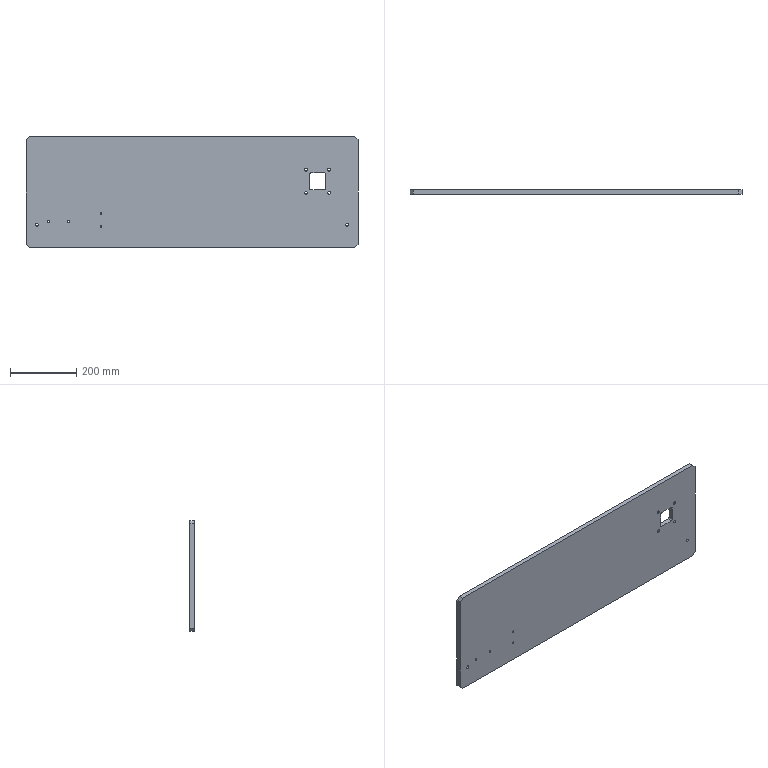Part | SolidWorks | features BaseBody 1 | 1 solid | 38 faces | box 1005 x 14 x 335 mm | volume 4668914 mm3 | cylinder 24 | plane 14 | commonest cylinder face diameters 8.5 x12 5 x4 6.8 x4 10 x4
STEP:
#1=CARTESIAN_POINT('',(470.,0.,-103.382));
#2=VERTEX_POINT('',#1);
#3=CARTESIAN_POINT('',(470.,0.,-94.882));
#4=VERTEX_POINT('',#3);
#5=CARTESIAN_POINT('',(470.,0.,-99.132));
#6=DIRECTION('',(0.,1.,0.));
#7=DIRECTION('',(0.,0.,1.));
#8=AXIS2_PLACEMENT_3D('',#5,#6,#7);
#9=CIRCLE('',#8,4.25);
#10=EDGE_CURVE('',#2,#4,#9,.T.);
#11=ORIENTED_EDGE('',*,*,#10,.F.);
#12=CARTESIAN_POINT('',(470.,14.,-103.382));
#13=VERTEX_POINT('',#12);
#14=CARTESIAN_POINT('',(470.,14.,-103.382));
#15=DIRECTION('',(0.,1.,0.));
#16=VECTOR('',#15,1000.);
#17=LINE('',#14,#16);
#18=EDGE_CURVE('',#2,#13,#17,.T.);
#19=ORIENTED_EDGE('',*,*,#18,.T.);
#20=CARTESIAN_POINT('',(470.,14.,-94.882));
#21=VERTEX_POINT('',#20);
#22=CARTESIAN_POINT('',(470.,14.,-99.132));
#23=DIRECTION('',(0.,1.,0.));
#24=DIRECTION('',(0.,0.,1.));
#25=AXIS2_PLACEMENT_3D('',#22,#23,#24);
#26=CIRCLE('',#25,4.25);
#27=EDGE_CURVE('',#13,#21,#26,.T.);
#28=ORIENTED_EDGE('',*,*,#27,.T.);
#29=CARTESIAN_POINT('',(470.,14.,-94.882));
#30=DIRECTION('',(0.,1.,0.));
#31=VECTOR('',#30,1000.);
#32=LINE('',#29,#31);
#33=EDGE_CURVE('',#4,#21,#32,.T.);
#34=ORIENTED_EDGE('',*,*,#33,.F.);
#35=EDGE_LOOP('',(#11,#19,#28,#34));
#36=FACE_OUTER_BOUND('',#35,.T.);
#37=CARTESIAN_POINT('',(470.,14.,-99.132));
#38=DIRECTION('',(0.,1.,0.));
#39=DIRECTION('',(0.,0.,1.));
#40=AXIS2_PLACEMENT_3D('',#37,#38,#39);
#41=CYLINDRICAL_SURFACE('',#40,4.25);
#42=ADVANCED_FACE('',(#36),#41,.F.);
#43=CARTESIAN_POINT('',(345.,0.,63.25));
#44=VERTEX_POINT('',#43);
#45=CARTESIAN_POINT('',(345.,0.,71.75));
#46=VERTEX_POINT('',#45);
#47=CARTESIAN_POINT('',(345.,0.,67.5));
#48=DIRECTION('',(0.,1.,0.));
#49=DIRECTION('',(0.,0.,1.));
#50=AXIS2_PLACEMENT_3D('',#47,#48,#49);
#51=CIRCLE('',#50,4.25);
#52=EDGE_CURVE('',#44,#46,#51,.T.);
#53=ORIENTED_EDGE('',*,*,#52,.F.);
#54=CARTESIAN_POINT('',(345.,14.,63.25));
#55=VERTEX_POINT('',#54);
#56=CARTESIAN_POINT('',(345.,14.,63.25));
#57=DIRECTION('',(0.,1.,0.));
#58=VECTOR('',#57,1000.);
#59=LINE('',#56,#58);
#60=EDGE_CURVE('',#44,#55,#59,.T.);
#61=ORIENTED_EDGE('',*,*,#60,.T.);
#62=CARTESIAN_POINT('',(345.,14.,71.75));
#63=VERTEX_POINT('',#62);
#64=CARTESIAN_POINT('',(345.,14.,67.5));
#65=DIRECTION('',(0.,1.,0.));
#66=DIRECTION('',(0.,0.,1.));
#67=AXIS2_PLACEMENT_3D('',#64,#65,#66);
#68=CIRCLE('',#67,4.25);
#69=EDGE_CURVE('',#55,#63,#68,.T.);
#70=ORIENTED_EDGE('',*,*,#69,.T.);
#71=CARTESIAN_POINT('',(345.,14.,71.75));
#72=DIRECTION('',(0.,1.,0.));
#73=VECTOR('',#72,1000.);
#74=LINE('',#71,#73);
#75=EDGE_CURVE('',#46,#63,#74,.T.);
#76=ORIENTED_EDGE('',*,*,#75,.F.);
#77=EDGE_LOOP('',(#53,#61,#70,#76));
#78=FACE_OUTER_BOUND('',#77,.T.);
#79=CARTESIAN_POINT('',(345.,14.,67.5));
#80=DIRECTION('',(0.,1.,0.));
#81=DIRECTION('',(0.,0.,1.));
#82=AXIS2_PLACEMENT_3D('',#79,#80,#81);
#83=CYLINDRICAL_SURFACE('',#82,4.25);
#84=ADVANCED_FACE('',(#78),#83,.F.);
#85=CARTESIAN_POINT('',(415.,0.,63.25));
#86=VERTEX_POINT('',#85);
#87=CARTESIAN_POINT('',(415.,0.,71.75));
#88=VERTEX_POINT('',#87);
#89=CARTESIAN_POINT('',(415.,0.,67.5));
#90=DIRECTION('',(0.,1.,0.));
#91=DIRECTION('',(0.,0.,1.));
#92=AXIS2_PLACEMENT_3D('',#89,#90,#91);
#93=CIRCLE('',#92,4.25);
#94=EDGE_CURVE('',#86,#88,#93,.T.);
#95=ORIENTED_EDGE('',*,*,#94,.F.);
#96=CARTESIAN_POINT('',(415.,14.,63.25));
#97=VERTEX_POINT('',#96);
#98=CARTESIAN_POINT('',(415.,14.,63.25));
#99=DIRECTION('',(0.,1.,0.));
#100=VECTOR('',#99,1000.);
#101=LINE('',#98,#100);
#102=EDGE_CURVE('',#86,#97,#101,.T.);
#103=ORIENTED_EDGE('',*,*,#102,.T.);
#104=CARTESIAN_POINT('',(415.,14.,71.75));
#105=VERTEX_POINT('',#104);
#106=CARTESIAN_POINT('',(415.,14.,67.5));
#107=DIRECTION('',(0.,1.,0.));
#108=DIRECTION('',(0.,0.,1.));
#109=AXIS2_PLACEMENT_3D('',#106,#107,#108);
#110=CIRCLE('',#109,4.25);
#111=EDGE_CURVE('',#97,#105,#110,.T.);
#112=ORIENTED_EDGE('',*,*,#111,.T.);
#113=CARTESIAN_POINT('',(415.,14.,71.75));
#114=DIRECTION('',(0.,1.,0.));
#115=VECTOR('',#114,1000.);
#116=LINE('',#113,#115);
#117=EDGE_CURVE('',#88,#105,#116,.T.);
#118=ORIENTED_EDGE('',*,*,#117,.F.);
#119=EDGE_LOOP('',(#95,#103,#112,#118));
#120=FACE_OUTER_BOUND('',#119,.T.);
#121=CARTESIAN_POINT('',(415.,14.,67.5));
#122=DIRECTION('',(0.,1.,0.));
#123=DIRECTION('',(0.,0.,1.));
#124=AXIS2_PLACEMENT_3D('',#121,#122,#123);
#125=CYLINDRICAL_SURFACE('',#124,4.25);
#126=ADVANCED_FACE('',(#120),#125,.F.);
#127=CARTESIAN_POINT('',(415.,0.,-6.75));
#128=VERTEX_POINT('',#127);
#129=CARTESIAN_POINT('',(415.,0.,1.75));
#130=VERTEX_POINT('',#129);
#131=CARTESIAN_POINT('',(415.,0.,-2.5));
#132=DIRECTION('',(0.,1.,0.));
#133=DIRECTION('',(0.,0.,1.));
#134=AXIS2_PLACEMENT_3D('',#131,#132,#133);
#135=CIRCLE('',#134,4.25);
#136=EDGE_CURVE('',#128,#130,#135,.T.);
#137=ORIENTED_EDGE('',*,*,#136,.F.);
#138=CARTESIAN_POINT('',(415.,14.,-6.75));
#139=VERTEX_POINT('',#138);
#140=CARTESIAN_POINT('',(415.,14.,-6.75));
#141=DIRECTION('',(0.,1.,0.));
#142=VECTOR('',#141,1000.);
#143=LINE('',#140,#142);
#144=EDGE_CURVE('',#128,#139,#143,.T.);
#145=ORIENTED_EDGE('',*,*,#144,.T.);
#146=CARTESIAN_POINT('',(415.,14.,1.75));
#147=VERTEX_POINT('',#146);
#148=CARTESIAN_POINT('',(415.,14.,-2.5));
#149=DIRECTION('',(0.,1.,0.));
#150=DIRECTION('',(0.,0.,1.));
#151=AXIS2_PLACEMENT_3D('',#148,#149,#150);
#152=CIRCLE('',#151,4.25);
#153=EDGE_CURVE('',#139,#147,#152,.T.);
#154=ORIENTED_EDGE('',*,*,#153,.T.);
#155=CARTESIAN_POINT('',(415.,14.,1.75));
#156=DIRECTION('',(0.,1.,0.));
#157=VECTOR('',#156,1000.);
#158=LINE('',#155,#157);
#159=EDGE_CURVE('',#130,#147,#158,.T.);
#160=ORIENTED_EDGE('',*,*,#159,.F.);
#161=EDGE_LOOP('',(#137,#145,#154,#160));
#162=FACE_OUTER_BOUND('',#161,.T.);
#163=CARTESIAN_POINT('',(415.,14.,-2.5));
#164=DIRECTION('',(0.,1.,0.));
#165=DIRECTION('',(0.,0.,1.));
#166=AXIS2_PLACEMENT_3D('',#163,#164,#165);
#167=CYLINDRICAL_SURFACE('',#166,4.25);
#168=ADVANCED_FACE('',(#162),#167,.F.);
#169=CARTESIAN_POINT('',(345.,0.,-6.75));
#170=VERTEX_POINT('',#169);
#171=CARTESIAN_POINT('',(345.,0.,1.75));
#172=VERTEX_POINT('',#171);
#173=CARTESIAN_POINT('',(345.,0.,-2.5));
#174=DIRECTION('',(0.,1.,0.));
#175=DIRECTION('',(0.,0.,1.));
#176=AXIS2_PLACEMENT_3D('',#173,#174,#175);
#177=CIRCLE('',#176,4.25);
#178=EDGE_CURVE('',#170,#172,#177,.T.);
#179=ORIENTED_EDGE('',*,*,#178,.F.);
#180=CARTESIAN_POINT('',(345.,14.,-6.75));
#181=VERTEX_POINT('',#180);
#182=CARTESIAN_POINT('',(345.,14.,-6.75));
#183=DIRECTION('',(0.,1.,0.));
#184=VECTOR('',#183,1000.);
#185=LINE('',#182,#184);
#186=EDGE_CURVE('',#170,#181,#185,.T.);
#187=ORIENTED_EDGE('',*,*,#186,.T.);
#188=CARTESIAN_POINT('',(345.,14.,1.75));
#189=VERTEX_POINT('',#188);
#190=CARTESIAN_POINT('',(345.,14.,-2.5));
#191=DIRECTION('',(0.,1.,0.));
#192=DIRECTION('',(0.,0.,1.));
#193=AXIS2_PLACEMENT_3D('',#190,#191,#192);
#194=CIRCLE('',#193,4.25);
#195=EDGE_CURVE('',#181,#189,#194,.T.);
#196=ORIENTED_EDGE('',*,*,#195,.T.);
#197=CARTESIAN_POINT('',(345.,14.,1.75));
#198=DIRECTION('',(0.,1.,0.));
#199=VECTOR('',#198,1000.);
#200=LINE('',#197,#199);
#201=EDGE_CURVE('',#172,#189,#200,.T.);
#202=ORIENTED_EDGE('',*,*,#201,.F.);
#203=EDGE_LOOP('',(#179,#187,#196,#202));
#204=FACE_OUTER_BOUND('',#203,.T.);
#205=CARTESIAN_POINT('',(345.,14.,-2.5));
#206=DIRECTION('',(0.,1.,0.));
#207=DIRECTION('',(0.,0.,1.));
#208=AXIS2_PLACEMENT_3D('',#205,#206,#207);
#209=CYLINDRICAL_SURFACE('',#208,4.25);
#210=ADVANCED_FACE('',(#204),#209,.F.);
#211=CARTESIAN_POINT('',(-470.,0.,-103.382));
#212=VERTEX_POINT('',#211);
#213=CARTESIAN_POINT('',(-470.,0.,-94.882));
#214=VERTEX_POINT('',#213);
#215=CARTESIAN_POINT('',(-470.,0.,-99.132));
#216=DIRECTION('',(0.,1.,0.));
#217=DIRECTION('',(0.,0.,1.));
#218=AXIS2_PLACEMENT_3D('',#215,#216,#217);
#219=CIRCLE('',#218,4.25);
#220=EDGE_CURVE('',#212,#214,#219,.T.);
#221=ORIENTED_EDGE('',*,*,#220,.F.);
#222=CARTESIAN_POINT('',(-470.,14.,-103.382));
#223=VERTEX_POINT('',#222);
#224=CARTESIAN_POINT('',(-470.,14.,-103.382));
#225=DIRECTION('',(0.,1.,0.));
#226=VECTOR('',#225,1000.);
#227=LINE('',#224,#226);
#228=EDGE_CURVE('',#212,#223,#227,.T.);
#229=ORIENTED_EDGE('',*,*,#228,.T.);
#230=CARTESIAN_POINT('',(-470.,14.,-94.882));
#231=VERTEX_POINT('',#230);
#232=CARTESIAN_POINT('',(-470.,14.,-99.132));
#233=DIRECTION('',(0.,1.,0.));
#234=DIRECTION('',(0.,0.,1.));
#235=AXIS2_PLACEMENT_3D('',#232,#233,#234);
#236=CIRCLE('',#235,4.25);
#237=EDGE_CURVE('',#223,#231,#236,.T.);
#238=ORIENTED_EDGE('',*,*,#237,.T.);
#239=CARTESIAN_POINT('',(-470.,14.,-94.882));
#240=DIRECTION('',(0.,1.,0.));
#241=VECTOR('',#240,1000.);
#242=LINE('',#239,#241);
#243=EDGE_CURVE('',#214,#231,#242,.T.);
#244=ORIENTED_EDGE('',*,*,#243,.F.);
#245=EDGE_LOOP('',(#221,#229,#238,#244));
#246=FACE_OUTER_BOUND('',#245,.T.);
#247=CARTESIAN_POINT('',(-470.,14.,-99.132));
#248=DIRECTION('',(0.,1.,0.));
#249=DIRECTION('',(0.,0.,1.));
#250=AXIS2_PLACEMENT_3D('',#247,#248,#249);
#251=CYLINDRICAL_SURFACE('',#250,4.25);
#252=ADVANCED_FACE('',(#246),#251,.F.);
#253=CARTESIAN_POINT('',(-375.,0.,-92.4));
#254=VERTEX_POINT('',#253);
#255=CARTESIAN_POINT('',(-375.,0.,-85.6));
#256=VERTEX_POINT('',#255);
#257=CARTESIAN_POINT('',(-375.,0.,-89.));
#258=DIRECTION('',(0.,1.,0.));
#259=DIRECTION('',(0.,0.,1.));
#260=AXIS2_PLACEMENT_3D('',#257,#258,#259);
#261=CIRCLE('',#260,3.4);
#262=EDGE_CURVE('',#254,#256,#261,.T.);
#263=ORIENTED_EDGE('',*,*,#262,.F.);
#264=CARTESIAN_POINT('',(-375.,14.,-92.4));
#265=VERTEX_POINT('',#264);
#266=CARTESIAN_POINT('',(-375.,14.,-92.4));
#267=DIRECTION('',(0.,1.,0.));
#268=VECTOR('',#267,1000.);
#269=LINE('',#266,#268);
#270=EDGE_CURVE('',#254,#265,#269,.T.);
#271=ORIENTED_EDGE('',*,*,#270,.T.);
#272=CARTESIAN_POINT('',(-375.,14.,-85.6));
#273=VERTEX_POINT('',#272);
#274=CARTESIAN_POINT('',(-375.,14.,-89.));
#275=DIRECTION('',(0.,1.,0.));
#276=DIRECTION('',(0.,0.,1.));
#277=AXIS2_PLACEMENT_3D('',#274,#275,#276);
#278=CIRCLE('',#277,3.4);
#279=EDGE_CURVE('',#265,#273,#278,.T.);
#280=ORIENTED_EDGE('',*,*,#279,.T.);
#281=CARTESIAN_POINT('',(-375.,14.,-85.6));
#282=DIRECTION('',(0.,1.,0.));
#283=VECTOR('',#282,1000.);
#284=LINE('',#281,#283);
#285=EDGE_CURVE('',#256,#273,#284,.T.);
#286=ORIENTED_EDGE('',*,*,#285,.F.);
#287=EDGE_LOOP('',(#263,#271,#280,#286));
#288=FACE_OUTER_BOUND('',#287,.T.);
#289=CARTESIAN_POINT('',(-375.,14.,-89.));
#290=DIRECTION('',(0.,1.,0.));
#291=DIRECTION('',(0.,0.,1.));
#292=AXIS2_PLACEMENT_3D('',#289,#290,#291);
#293=CYLINDRICAL_SURFACE('',#292,3.4);
#294=ADVANCED_FACE('',(#288),#293,.F.);
#295=CARTESIAN_POINT('',(-435.,0.,-92.4));
#296=VERTEX_POINT('',#295);
#297=CARTESIAN_POINT('',(-435.,0.,-85.6));
#298=VERTEX_POINT('',#297);
#299=CARTESIAN_POINT('',(-435.,0.,-89.));
#300=DIRECTION('',(0.,1.,0.));
#301=DIRECTION('',(0.,0.,1.));
#302=AXIS2_PLACEMENT_3D('',#299,#300,#301);
#303=CIRCLE('',#302,3.4);
#304=EDGE_CURVE('',#296,#298,#303,.T.);
#305=ORIENTED_EDGE('',*,*,#304,.F.);
#306=CARTESIAN_POINT('',(-435.,14.,-92.4));
#307=VERTEX_POINT('',#306);
#308=CARTESIAN_POINT('',(-435.,14.,-92.4));
#309=DIRECTION('',(0.,1.,0.));
#310=VECTOR('',#309,1000.);
#311=LINE('',#308,#310);
#312=EDGE_CURVE('',#296,#307,#311,.T.);
#313=ORIENTED_EDGE('',*,*,#312,.T.);
#314=CARTESIAN_POINT('',(-435.,14.,-85.6));
#315=VERTEX_POINT('',#314);
#316=CARTESIAN_POINT('',(-435.,14.,-89.));
#317=DIRECTION('',(0.,1.,0.));
#318=DIRECTION('',(0.,0.,1.));
#319=AXIS2_PLACEMENT_3D('',#316,#317,#318);
#320=CIRCLE('',#319,3.4);
#321=EDGE_CURVE('',#307,#315,#320,.T.);
#322=ORIENTED_EDGE('',*,*,#321,.T.);
#323=CARTESIAN_POINT('',(-435.,14.,-85.6));
#324=DIRECTION('',(0.,1.,0.));
#325=VECTOR('',#324,1000.);
#326=LINE('',#323,#325);
#327=EDGE_CURVE('',#298,#315,#326,.T.);
#328=ORIENTED_EDGE('',*,*,#327,.F.);
#329=EDGE_LOOP('',(#305,#313,#322,#328));
#330=FACE_OUTER_BOUND('',#329,.T.);
#331=CARTESIAN_POINT('',(-435.,14.,-89.));
#332=DIRECTION('',(0.,1.,0.));
#333=DIRECTION('',(0.,0.,1.));
#334=AXIS2_PLACEMENT_3D('',#331,#332,#333);
#335=CYLINDRICAL_SURFACE('',#334,3.4);
#336=ADVANCED_FACE('',(#330),#335,.F.);
#337=CARTESIAN_POINT('',(-275.5,0.,-67.));
#338=VERTEX_POINT('',#337);
#339=CARTESIAN_POINT('',(-275.5,0.,-62.));
#340=VERTEX_POINT('',#339);
#341=CARTESIAN_POINT('',(-275.5,0.,-64.5));
#342=DIRECTION('',(0.,1.,0.));
#343=DIRECTION('',(0.,0.,1.));
#344=AXIS2_PLACEMENT_3D('',#341,#342,#343);
#345=CIRCLE('',#344,2.5);
#346=EDGE_CURVE('',#338,#340,#345,.T.);
#347=ORIENTED_EDGE('',*,*,#346,.F.);
#348=CARTESIAN_POINT('',(-275.5,14.,-67.));
#349=VERTEX_POINT('',#348);
#350=CARTESIAN_POINT('',(-275.5,14.,-67.));
#351=DIRECTION('',(0.,1.,0.));
#352=VECTOR('',#351,1000.);
#353=LINE('',#350,#352);
#354=EDGE_CURVE('',#338,#349,#353,.T.);
#355=ORIENTED_EDGE('',*,*,#354,.T.);
#356=CARTESIAN_POINT('',(-275.5,14.,-62.));
#357=VERTEX_POINT('',#356);
#358=CARTESIAN_POINT('',(-275.5,14.,-64.5));
#359=DIRECTION('',(0.,1.,0.));
#360=DIRECTION('',(0.,0.,1.));
#361=AXIS2_PLACEMENT_3D('',#358,#359,#360);
#362=CIRCLE('',#361,2.5);
#363=EDGE_CURVE('',#349,#357,#362,.T.);
#364=ORIENTED_EDGE('',*,*,#363,.T.);
#365=CARTESIAN_POINT('',(-275.5,14.,-62.));
#366=DIRECTION('',(0.,1.,0.));
#367=VECTOR('',#366,1000.);
#368=LINE('',#365,#367);
#369=EDGE_CURVE('',#340,#357,#368,.T.);
#370=ORIENTED_EDGE('',*,*,#369,.F.);
#371=EDGE_LOOP('',(#347,#355,#364,#370));
#372=FACE_OUTER_BOUND('',#371,.T.);
#373=CARTESIAN_POINT('',(-275.5,14.,-64.5));
#374=DIRECTION('',(0.,1.,0.));
#375=DIRECTION('',(0.,0.,1.));
#376=AXIS2_PLACEMENT_3D('',#373,#374,#375);
#377=CYLINDRICAL_SURFACE('',#376,2.5);
#378=ADVANCED_FACE('',(#372),#377,.F.);
#379=CARTESIAN_POINT('',(-275.5,0.,-107.));
#380=VERTEX_POINT('',#379);
#381=CARTESIAN_POINT('',(-275.5,0.,-102.));
#382=VERTEX_POINT('',#381);
#383=CARTESIAN_POINT('',(-275.5,0.,-104.5));
#384=DIRECTION('',(0.,1.,0.));
#385=DIRECTION('',(0.,0.,1.));
#386=AXIS2_PLACEMENT_3D('',#383,#384,#385);
#387=CIRCLE('',#386,2.5);
#388=EDGE_CURVE('',#380,#382,#387,.T.);
#389=ORIENTED_EDGE('',*,*,#388,.F.);
#390=CARTESIAN_POINT('',(-275.5,14.,-107.));
#391=VERTEX_POINT('',#390);
#392=CARTESIAN_POINT('',(-275.5,14.,-107.));
#393=DIRECTION('',(0.,1.,0.));
#394=VECTOR('',#393,1000.);
#395=LINE('',#392,#394);
#396=EDGE_CURVE('',#380,#391,#395,.T.);
#397=ORIENTED_EDGE('',*,*,#396,.T.);
#398=CARTESIAN_POINT('',(-275.5,14.,-102.));
#399=VERTEX_POINT('',#398);
#400=CARTESIAN_POINT('',(-275.5,14.,-104.5));
#401=DIRECTION('',(0.,1.,0.));
#402=DIRECTION('',(0.,0.,1.));
#403=AXIS2_PLACEMENT_3D('',#400,#401,#402);
#404=CIRCLE('',#403,2.5);
#405=EDGE_CURVE('',#391,#399,#404,.T.);
#406=ORIENTED_EDGE('',*,*,#405,.T.);
#407=CARTESIAN_POINT('',(-275.5,14.,-102.));
#408=DIRECTION('',(0.,1.,0.));
#409=VECTOR('',#408,1000.);
#410=LINE('',#407,#409);
#411=EDGE_CURVE('',#382,#399,#410,.T.);
#412=ORIENTED_EDGE('',*,*,#411,.F.);
#413=EDGE_LOOP('',(#389,#397,#406,#412));
#414=FACE_OUTER_BOUND('',#413,.T.);
#415=CARTESIAN_POINT('',(-275.5,14.,-104.5));
#416=DIRECTION('',(0.,1.,0.));
#417=DIRECTION('',(0.,0.,1.));
#418=AXIS2_PLACEMENT_3D('',#415,#416,#417);
#419=CYLINDRICAL_SURFACE('',#418,2.5);
#420=ADVANCED_FACE('',(#414),#419,.F.);
#421=CARTESIAN_POINT('',(-492.5,14.,167.5));
#422=VERTEX_POINT('',#421);
#423=CARTESIAN_POINT('',(-502.5,14.,157.5));
#424=VERTEX_POINT('',#423);
#425=CARTESIAN_POINT('',(-492.5,14.,167.5));
#426=DIRECTION('',(-0.7071,0.,-0.7071));
#427=VECTOR('',#426,1000.);
#428=LINE('',#425,#427);
#429=EDGE_CURVE('',#422,#424,#428,.T.);
#430=ORIENTED_EDGE('',*,*,#429,.F.);
#431=CARTESIAN_POINT('',(492.5,14.,167.5));
#432=VERTEX_POINT('',#431);
#433=CARTESIAN_POINT('',(0.,14.,167.5));
#434=DIRECTION('',(-1.,0.,0.));
#435=VECTOR('',#434,1000.);
#436=LINE('',#433,#435);
#437=EDGE_CURVE('',#432,#422,#436,.T.);
#438=ORIENTED_EDGE('',*,*,#437,.F.);
#439=CARTESIAN_POINT('',(502.5,14.,157.5));
#440=VERTEX_POINT('',#439);
#441=CARTESIAN_POINT('',(502.5,14.,157.5));
#442=DIRECTION('',(-0.7071,0.,0.7071));
#443=VECTOR('',#442,1000.);
#444=LINE('',#441,#443);
#445=EDGE_CURVE('',#440,#432,#444,.T.);
#446=ORIENTED_EDGE('',*,*,#445,.F.);
#447=CARTESIAN_POINT('',(502.5,14.,-157.5));
#448=VERTEX_POINT('',#447);
#449=CARTESIAN_POINT('',(502.5,14.,0.));
#450=DIRECTION('',(0.,0.,1.));
#451=VECTOR('',#450,1000.);
#452=LINE('',#449,#451);
#453=EDGE_CURVE('',#448,#440,#452,.T.);
#454=ORIENTED_EDGE('',*,*,#453,.F.);
#455=CARTESIAN_POINT('',(492.5,14.,-167.5));
#456=VERTEX_POINT('',#455);
#457=CARTESIAN_POINT('',(492.5,14.,-167.5));
#458=DIRECTION('',(0.7071,0.,0.7071));
#459=VECTOR('',#458,1000.);
#460=LINE('',#457,#459);
#461=EDGE_CURVE('',#456,#448,#460,.T.);
#462=ORIENTED_EDGE('',*,*,#461,.F.);
#463=CARTESIAN_POINT('',(-492.5,14.,-167.5));
#464=VERTEX_POINT('',#463);
#465=CARTESIAN_POINT('',(0.,14.,-167.5));
#466=DIRECTION('',(1.,0.,0.));
#467=VECTOR('',#466,1000.);
#468=LINE('',#465,#467);
#469=EDGE_CURVE('',#464,#456,#468,.T.);
#470=ORIENTED_EDGE('',*,*,#469,.F.);
#471=CARTESIAN_POINT('',(-502.5,14.,-157.5));
#472=VERTEX_POINT('',#471);
#473=CARTESIAN_POINT('',(-502.5,14.,-157.5));
#474=DIRECTION('',(0.7071,0.,-0.7071));
#475=VECTOR('',#474,1000.);
#476=LINE('',#473,#475);
#477=EDGE_CURVE('',#472,#464,#476,.T.);
#478=ORIENTED_EDGE('',*,*,#477,.F.);
#479=CARTESIAN_POINT('',(-502.5,14.,0.));
#480=DIRECTION('',(0.,0.,-1.));
#481=VECTOR('',#480,1000.);
#482=LINE('',#479,#481);
#483=EDGE_CURVE('',#424,#472,#482,.T.);
#484=ORIENTED_EDGE('',*,*,#483,.F.);
#485=EDGE_LOOP('',(#430,#438,#446,#454,#462,#470,#478,#484));
#486=FACE_OUTER_BOUND('',#485,.T.);
#487=CARTESIAN_POINT('',(470.,14.,-99.132));
#488=DIRECTION('',(0.,1.,0.));
#489=DIRECTION('',(0.,0.,1.));
#490=AXIS2_PLACEMENT_3D('',#487,#488,#489);
#491=CIRCLE('',#490,4.25);
#492=EDGE_CURVE('',#21,#13,#491,.T.);
#493=ORIENTED_EDGE('',*,*,#492,.F.);
#494=ORIENTED_EDGE('',*,*,#27,.F.);
#495=EDGE_LOOP('',(#493,#494));
#496=FACE_BOUND('',#495,.T.);
#497=CARTESIAN_POINT('',(345.,14.,67.5));
#498=DIRECTION('',(0.,1.,0.));
#499=DIRECTION('',(0.,0.,1.));
#500=AXIS2_PLACEMENT_3D('',#497,#498,#499);
#501=CIRCLE('',#500,4.25);
#502=EDGE_CURVE('',#63,#55,#501,.T.);
#503=ORIENTED_EDGE('',*,*,#502,.F.);
#504=ORIENTED_EDGE('',*,*,#69,.F.);
#505=EDGE_LOOP('',(#503,#504));
#506=FACE_BOUND('',#505,.T.);
#507=CARTESIAN_POINT('',(415.,14.,67.5));
#508=DIRECTION('',(0.,1.,0.));
#509=DIRECTION('',(0.,0.,1.));
#510=AXIS2_PLACEMENT_3D('',#507,#508,#509);
#511=CIRCLE('',#510,4.25);
#512=EDGE_CURVE('',#105,#97,#511,.T.);
#513=ORIENTED_EDGE('',*,*,#512,.F.);
#514=ORIENTED_EDGE('',*,*,#111,.F.);
#515=EDGE_LOOP('',(#513,#514));
#516=FACE_BOUND('',#515,.T.);
#517=CARTESIAN_POINT('',(415.,14.,-2.5));
#518=DIRECTION('',(0.,1.,0.));
#519=DIRECTION('',(0.,0.,1.));
#520=AXIS2_PLACEMENT_3D('',#517,#518,#519);
#521=CIRCLE('',#520,4.25);
#522=EDGE_CURVE('',#147,#139,#521,.T.);
#523=ORIENTED_EDGE('',*,*,#522,.F.);
#524=ORIENTED_EDGE('',*,*,#153,.F.);
#525=EDGE_LOOP('',(#523,#524));
#526=FACE_BOUND('',#525,.T.);
#527=CARTESIAN_POINT('',(345.,14.,-2.5));
#528=DIRECTION('',(0.,1.,0.));
#529=DIRECTION('',(0.,0.,1.));
#530=AXIS2_PLACEMENT_3D('',#527,#528,#529);
#531=CIRCLE('',#530,4.25);
#532=EDGE_CURVE('',#189,#181,#531,.T.);
#533=ORIENTED_EDGE('',*,*,#532,.F.);
#534=ORIENTED_EDGE('',*,*,#195,.F.);
#535=EDGE_LOOP('',(#533,#534));
#536=FACE_BOUND('',#535,.T.);
#537=CARTESIAN_POINT('',(-470.,14.,-99.132));
#538=DIRECTION('',(0.,1.,0.));
#539=DIRECTION('',(0.,0.,1.));
#540=AXIS2_PLACEMENT_3D('',#537,#538,#539);
#541=CIRCLE('',#540,4.25);
#542=EDGE_CURVE('',#231,#223,#541,.T.);
#543=ORIENTED_EDGE('',*,*,#542,.F.);
#544=ORIENTED_EDGE('',*,*,#237,.F.);
#545=EDGE_LOOP('',(#543,#544));
#546=FACE_BOUND('',#545,.T.);
#547=CARTESIAN_POINT('',(-375.,14.,-89.));
#548=DIRECTION('',(0.,1.,0.));
#549=DIRECTION('',(0.,0.,1.));
#550=AXIS2_PLACEMENT_3D('',#547,#548,#549);
#551=CIRCLE('',#550,3.4);
#552=EDGE_CURVE('',#273,#265,#551,.T.);
#553=ORIENTED_EDGE('',*,*,#552,.F.);
#554=ORIENTED_EDGE('',*,*,#279,.F.);
#555=EDGE_LOOP('',(#553,#554));
#556=FACE_BOUND('',#555,.T.);
#557=CARTESIAN_POINT('',(-435.,14.,-89.));
#558=DIRECTION('',(0.,1.,0.));
#559=DIRECTION('',(0.,0.,1.));
#560=AXIS2_PLACEMENT_3D('',#557,#558,#559);
#561=CIRCLE('',#560,3.4);
#562=EDGE_CURVE('',#315,#307,#561,.T.);
#563=ORIENTED_EDGE('',*,*,#562,.F.);
#564=ORIENTED_EDGE('',*,*,#321,.F.);
#565=EDGE_LOOP('',(#563,#564));
#566=FACE_BOUND('',#565,.T.);
#567=CARTESIAN_POINT('',(360.,14.,7.45));
#568=VERTEX_POINT('',#567);
#569=CARTESIAN_POINT('',(355.,14.,12.45));
#570=VERTEX_POINT('',#569);
#571=CARTESIAN_POINT('',(360.,14.,12.45));
#572=DIRECTION('',(0.,1.,0.));
#573=DIRECTION('',(0.,0.,-1.));
#574=AXIS2_PLACEMENT_3D('',#571,#572,#573);
#575=CIRCLE('',#574,5.);
#576=EDGE_CURVE('',#568,#570,#575,.T.);
#577=ORIENTED_EDGE('',*,*,#576,.F.);
#578=CARTESIAN_POINT('',(400.5,14.,7.45));
#579=VERTEX_POINT('',#578);
#580=CARTESIAN_POINT('',(0.,14.,7.45));
#581=DIRECTION('',(-1.,0.,0.));
#582=VECTOR('',#581,1000.);
#583=LINE('',#580,#582);
#584=EDGE_CURVE('',#579,#568,#583,.T.);
#585=ORIENTED_EDGE('',*,*,#584,.F.);
#586=CARTESIAN_POINT('',(405.5,14.,12.45));
#587=VERTEX_POINT('',#586);
#588=CARTESIAN_POINT('',(400.5,14.,12.45));
#589=DIRECTION('',(0.,1.,0.));
#590=DIRECTION('',(0.,0.,-1.));
#591=AXIS2_PLACEMENT_3D('',#588,#589,#590);
#592=CIRCLE('',#591,5.);
#593=EDGE_CURVE('',#587,#579,#592,.T.);
#594=ORIENTED_EDGE('',*,*,#593,.F.);
#595=CARTESIAN_POINT('',(405.5,14.,52.95));
#596=VERTEX_POINT('',#595);
#597=CARTESIAN_POINT('',(405.5,14.,0.));
#598=DIRECTION('',(0.,0.,-1.));
#599=VECTOR('',#598,1000.);
#600=LINE('',#597,#599);
#601=EDGE_CURVE('',#596,#587,#600,.T.);
#602=ORIENTED_EDGE('',*,*,#601,.F.);
#603=CARTESIAN_POINT('',(400.5,14.,57.95));
#604=VERTEX_POINT('',#603);
#605=CARTESIAN_POINT('',(400.5,14.,52.95));
#606=DIRECTION('',(0.,1.,0.));
#607=DIRECTION('',(0.,0.,-1.));
#608=AXIS2_PLACEMENT_3D('',#605,#606,#607);
#609=CIRCLE('',#608,5.);
#610=EDGE_CURVE('',#604,#596,#609,.T.);
#611=ORIENTED_EDGE('',*,*,#610,.F.);
#612=CARTESIAN_POINT('',(360.,14.,57.95));
#613=VERTEX_POINT('',#612);
#614=CARTESIAN_POINT('',(0.,14.,57.95));
#615=DIRECTION('',(1.,0.,0.));
#616=VECTOR('',#615,1000.);
#617=LINE('',#614,#616);
#618=EDGE_CURVE('',#613,#604,#617,.T.);
#619=ORIENTED_EDGE('',*,*,#618,.F.);
#620=CARTESIAN_POINT('',(355.,14.,52.95));
#621=VERTEX_POINT('',#620);
#622=CARTESIAN_POINT('',(360.,14.,52.95));
#623=DIRECTION('',(0.,1.,0.));
#624=DIRECTION('',(0.,0.,-1.));
#625=AXIS2_PLACEMENT_3D('',#622,#623,#624);
#626=CIRCLE('',#625,5.);
#627=EDGE_CURVE('',#621,#613,#626,.T.);
#628=ORIENTED_EDGE('',*,*,#627,.F.);
#629=CARTESIAN_POINT('',(355.,14.,0.));
#630=DIRECTION('',(0.,0.,1.));
#631=VECTOR('',#630,1000.);
#632=LINE('',#629,#631);
#633=EDGE_CURVE('',#570,#621,#632,.T.);
#634=ORIENTED_EDGE('',*,*,#633,.F.);
#635=EDGE_LOOP('',(#577,#585,#594,#602,#611,#619,#628,#634));
#636=FACE_BOUND('',#635,.T.);
#637=CARTESIAN_POINT('',(-275.5,14.,-64.5));
#638=DIRECTION('',(0.,1.,0.));
#639=DIRECTION('',(0.,0.,1.));
#640=AXIS2_PLACEMENT_3D('',#637,#638,#639);
#641=CIRCLE('',#640,2.5);
#642=EDGE_CURVE('',#357,#349,#641,.T.);
#643=ORIENTED_EDGE('',*,*,#642,.F.);
#644=ORIENTED_EDGE('',*,*,#363,.F.);
#645=EDGE_LOOP('',(#643,#644));
#646=FACE_BOUND('',#645,.T.);
#647=CARTESIAN_POINT('',(-275.5,14.,-104.5));
#648=DIRECTION('',(0.,1.,0.));
#649=DIRECTION('',(0.,0.,1.));
#650=AXIS2_PLACEMENT_3D('',#647,#648,#649);
#651=CIRCLE('',#650,2.5);
#652=EDGE_CURVE('',#399,#391,#651,.T.);
#653=ORIENTED_EDGE('',*,*,#652,.F.);
#654=ORIENTED_EDGE('',*,*,#405,.F.);
#655=EDGE_LOOP('',(#653,#654));
#656=FACE_BOUND('',#655,.T.);
#657=CARTESIAN_POINT('',(0.,14.,0.));
#658=DIRECTION('',(0.,-1.,0.));
#659=DIRECTION('',(0.,0.,-1.));
#660=AXIS2_PLACEMENT_3D('',#657,#658,#659);
#661=PLANE('',#660);
#662=ADVANCED_FACE('',(#486,#496,#506,#516,#526,#536,#546,#556,#566,#636,#646,#656),#661,.F.);
#663=CARTESIAN_POINT('',(-502.5,0.,157.5));
#664=VERTEX_POINT('',#663);
#665=CARTESIAN_POINT('',(-502.5,14.,157.5));
#666=DIRECTION('',(0.,-1.,0.));
#667=VECTOR('',#666,1000.);
#668=LINE('',#665,#667);
#669=EDGE_CURVE('',#424,#664,#668,.T.);
#670=ORIENTED_EDGE('',*,*,#669,.F.);
#671=ORIENTED_EDGE('',*,*,#483,.T.);
#672=CARTESIAN_POINT('',(-502.5,0.,-157.5));
#673=VERTEX_POINT('',#672);
#674=CARTESIAN_POINT('',(-502.5,14.,-157.5));
#675=DIRECTION('',(0.,1.,0.));
#676=VECTOR('',#675,1000.);
#677=LINE('',#674,#676);
#678=EDGE_CURVE('',#673,#472,#677,.T.);
#679=ORIENTED_EDGE('',*,*,#678,.F.);
#680=CARTESIAN_POINT('',(-502.5,0.,167.5));
#681=DIRECTION('',(0.,0.,-1.));
#682=VECTOR('',#681,1000.);
#683=LINE('',#680,#682);
#684=EDGE_CURVE('',#664,#673,#683,.T.);
#685=ORIENTED_EDGE('',*,*,#684,.F.);
#686=EDGE_LOOP('',(#670,#671,#679,#685));
#687=FACE_OUTER_BOUND('',#686,.T.);
#688=CARTESIAN_POINT('',(-502.5,14.,167.5));
#689=DIRECTION('',(1.,0.,0.));
#690=DIRECTION('',(0.,0.,-1.));
#691=AXIS2_PLACEMENT_3D('',#688,#689,#690);
#692=PLANE('',#691);
#693=ADVANCED_FACE('',(#687),#692,.F.);
#694=ORIENTED_EDGE('',*,*,#669,.T.);
#695=CARTESIAN_POINT('',(-492.5,0.,167.5));
#696=VERTEX_POINT('',#695);
#697=CARTESIAN_POINT('',(-492.5,0.,167.5));
#698=DIRECTION('',(-0.7071,0.,-0.7071));
#699=VECTOR('',#698,1000.);
#700=LINE('',#697,#699);
#701=EDGE_CURVE('',#696,#664,#700,.T.);
#702=ORIENTED_EDGE('',*,*,#701,.F.);
#703=CARTESIAN_POINT('',(-492.5,14.,167.5));
#704=DIRECTION('',(0.,-1.,0.));
#705=VECTOR('',#704,1000.);
#706=LINE('',#703,#705);
#707=EDGE_CURVE('',#422,#696,#706,.T.);
#708=ORIENTED_EDGE('',*,*,#707,.F.);
#709=ORIENTED_EDGE('',*,*,#429,.T.);
#710=EDGE_LOOP('',(#694,#702,#708,#709));
#711=FACE_OUTER_BOUND('',#710,.T.);
#712=CARTESIAN_POINT('',(-492.5,14.,167.5));
#713=DIRECTION('',(0.7071,0.,-0.7071));
#714=DIRECTION('',(-0.7071,0.,-0.7071));
#715=AXIS2_PLACEMENT_3D('',#712,#713,#714);
#716=PLANE('',#715);
#717=ADVANCED_FACE('',(#711),#716,.F.);
#718=ORIENTED_EDGE('',*,*,#707,.T.);
#719=CARTESIAN_POINT('',(492.5,0.,167.5));
#720=VERTEX_POINT('',#719);
#721=CARTESIAN_POINT('',(-502.5,0.,167.5));
#722=DIRECTION('',(-1.,0.,0.));
#723=VECTOR('',#722,1000.);
#724=LINE('',#721,#723);
#725=EDGE_CURVE('',#720,#696,#724,.T.);
#726=ORIENTED_EDGE('',*,*,#725,.F.);
#727=CARTESIAN_POINT('',(492.5,14.,167.5));
#728=DIRECTION('',(0.,-1.,0.));
#729=VECTOR('',#728,1000.);
#730=LINE('',#727,#729);
#731=EDGE_CURVE('',#432,#720,#730,.T.);
#732=ORIENTED_EDGE('',*,*,#731,.F.);
#733=ORIENTED_EDGE('',*,*,#437,.T.);
#734=EDGE_LOOP('',(#718,#726,#732,#733));
#735=FACE_OUTER_BOUND('',#734,.T.);
#736=CARTESIAN_POINT('',(-502.5,14.,167.5));
#737=DIRECTION('',(0.,0.,-1.));
#738=DIRECTION('',(-1.,0.,0.));
#739=AXIS2_PLACEMENT_3D('',#736,#737,#738);
#740=PLANE('',#739);
#741=ADVANCED_FACE('',(#735),#740,.F.);
#742=ORIENTED_EDGE('',*,*,#731,.T.);
#743=CARTESIAN_POINT('',(502.5,0.,157.5));
#744=VERTEX_POINT('',#743);
#745=CARTESIAN_POINT('',(502.5,0.,157.5));
#746=DIRECTION('',(-0.7071,0.,0.7071));
#747=VECTOR('',#746,1000.);
#748=LINE('',#745,#747);
#749=EDGE_CURVE('',#744,#720,#748,.T.);
#750=ORIENTED_EDGE('',*,*,#749,.F.);
#751=CARTESIAN_POINT('',(502.5,14.,157.5));
#752=DIRECTION('',(0.,-1.,0.));
#753=VECTOR('',#752,1000.);
#754=LINE('',#751,#753);
#755=EDGE_CURVE('',#440,#744,#754,.T.);
#756=ORIENTED_EDGE('',*,*,#755,.F.);
#757=ORIENTED_EDGE('',*,*,#445,.T.);
#758=EDGE_LOOP('',(#742,#750,#756,#757));
#759=FACE_OUTER_BOUND('',#758,.T.);
#760=CARTESIAN_POINT('',(502.5,14.,157.5));
#761=DIRECTION('',(-0.7071,0.,-0.7071));
#762=DIRECTION('',(-0.7071,0.,0.7071));
#763=AXIS2_PLACEMENT_3D('',#760,#761,#762);
#764=PLANE('',#763);
#765=ADVANCED_FACE('',(#759),#764,.F.);
#766=ORIENTED_EDGE('',*,*,#755,.T.);
#767=CARTESIAN_POINT('',(502.5,0.,-157.5));
#768=VERTEX_POINT('',#767);
#769=CARTESIAN_POINT('',(502.5,0.,167.5));
#770=DIRECTION('',(0.,0.,1.));
#771=VECTOR('',#770,1000.);
#772=LINE('',#769,#771);
#773=EDGE_CURVE('',#768,#744,#772,.T.);
#774=ORIENTED_EDGE('',*,*,#773,.F.);
#775=CARTESIAN_POINT('',(502.5,14.,-157.5));
#776=DIRECTION('',(0.,-1.,0.));
#777=VECTOR('',#776,1000.);
#778=LINE('',#775,#777);
#779=EDGE_CURVE('',#448,#768,#778,.T.);
#780=ORIENTED_EDGE('',*,*,#779,.F.);
#781=ORIENTED_EDGE('',*,*,#453,.T.);
#782=EDGE_LOOP('',(#766,#774,#780,#781));
#783=FACE_OUTER_BOUND('',#782,.T.);
#784=CARTESIAN_POINT('',(502.5,14.,167.5));
#785=DIRECTION('',(-1.,0.,0.));
#786=DIRECTION('',(0.,0.,1.));
#787=AXIS2_PLACEMENT_3D('',#784,#785,#786);
#788=PLANE('',#787);
#789=ADVANCED_FACE('',(#783),#788,.F.);
#790=ORIENTED_EDGE('',*,*,#779,.T.);
#791=CARTESIAN_POINT('',(492.5,0.,-167.5));
#792=VERTEX_POINT('',#791);
#793=CARTESIAN_POINT('',(492.5,0.,-167.5));
#794=DIRECTION('',(0.7071,0.,0.7071));
#795=VECTOR('',#794,1000.);
#796=LINE('',#793,#795);
#797=EDGE_CURVE('',#792,#768,#796,.T.);
#798=ORIENTED_EDGE('',*,*,#797,.F.);
#799=CARTESIAN_POINT('',(492.5,14.,-167.5));
#800=DIRECTION('',(0.,-1.,0.));
#801=VECTOR('',#800,1000.);
#802=LINE('',#799,#801);
#803=EDGE_CURVE('',#456,#792,#802,.T.);
#804=ORIENTED_EDGE('',*,*,#803,.F.);
#805=ORIENTED_EDGE('',*,*,#461,.T.);
#806=EDGE_LOOP('',(#790,#798,#804,#805));
#807=FACE_OUTER_BOUND('',#806,.T.);
#808=CARTESIAN_POINT('',(492.5,14.,-167.5));
#809=DIRECTION('',(-0.7071,0.,0.7071));
#810=DIRECTION('',(0.7071,0.,0.7071));
#811=AXIS2_PLACEMENT_3D('',#808,#809,#810);
#812=PLANE('',#811);
#813=ADVANCED_FACE('',(#807),#812,.F.);
#814=ORIENTED_EDGE('',*,*,#803,.T.);
#815=CARTESIAN_POINT('',(-492.5,0.,-167.5));
#816=VERTEX_POINT('',#815);
#817=CARTESIAN_POINT('',(-502.5,0.,-167.5));
#818=DIRECTION('',(1.,0.,0.));
#819=VECTOR('',#818,1000.);
#820=LINE('',#817,#819);
#821=EDGE_CURVE('',#816,#792,#820,.T.);
#822=ORIENTED_EDGE('',*,*,#821,.F.);
#823=CARTESIAN_POINT('',(-492.5,14.,-167.5));
#824=DIRECTION('',(0.,-1.,0.));
#825=VECTOR('',#824,1000.);
#826=LINE('',#823,#825);
#827=EDGE_CURVE('',#464,#816,#826,.T.);
#828=ORIENTED_EDGE('',*,*,#827,.F.);
#829=ORIENTED_EDGE('',*,*,#469,.T.);
#830=EDGE_LOOP('',(#814,#822,#828,#829));
#831=FACE_OUTER_BOUND('',#830,.T.);
#832=CARTESIAN_POINT('',(-502.5,14.,-167.5));
#833=DIRECTION('',(0.,0.,1.));
#834=DIRECTION('',(1.,0.,0.));
#835=AXIS2_PLACEMENT_3D('',#832,#833,#834);
#836=PLANE('',#835);
#837=ADVANCED_FACE('',(#831),#836,.F.);
#838=ORIENTED_EDGE('',*,*,#827,.T.);
#839=CARTESIAN_POINT('',(-502.5,0.,-157.5));
#840=DIRECTION('',(0.7071,0.,-0.7071));
#841=VECTOR('',#840,1000.);
#842=LINE('',#839,#841);
#843=EDGE_CURVE('',#673,#816,#842,.T.);
#844=ORIENTED_EDGE('',*,*,#843,.F.);
#845=ORIENTED_EDGE('',*,*,#678,.T.);
#846=ORIENTED_EDGE('',*,*,#477,.T.);
#847=EDGE_LOOP('',(#838,#844,#845,#846));
#848=FACE_OUTER_BOUND('',#847,.T.);
#849=CARTESIAN_POINT('',(-502.5,14.,-157.5));
#850=DIRECTION('',(0.7071,0.,0.7071));
#851=DIRECTION('',(0.7071,0.,-0.7071));
#852=AXIS2_PLACEMENT_3D('',#849,#850,#851);
#853=PLANE('',#852);
#854=ADVANCED_FACE('',(#848),#853,.F.);
#855=ORIENTED_EDGE('',*,*,#18,.F.);
#856=CARTESIAN_POINT('',(470.,0.,-99.132));
#857=DIRECTION('',(0.,1.,0.));
#858=DIRECTION('',(0.,0.,1.));
#859=AXIS2_PLACEMENT_3D('',#856,#857,#858);
#860=CIRCLE('',#859,4.25);
#861=EDGE_CURVE('',#4,#2,#860,.T.);
#862=ORIENTED_EDGE('',*,*,#861,.F.);
#863=ORIENTED_EDGE('',*,*,#33,.T.);
#864=ORIENTED_EDGE('',*,*,#492,.T.);
#865=EDGE_LOOP('',(#855,#862,#863,#864));
#866=FACE_OUTER_BOUND('',#865,.T.);
#867=CARTESIAN_POINT('',(470.,14.,-99.132));
#868=DIRECTION('',(0.,1.,0.));
#869=DIRECTION('',(0.,0.,1.));
#870=AXIS2_PLACEMENT_3D('',#867,#868,#869);
#871=CYLINDRICAL_SURFACE('',#870,4.25);
#872=ADVANCED_FACE('',(#866),#871,.F.);
#873=ORIENTED_EDGE('',*,*,#60,.F.);
#874=CARTESIAN_POINT('',(345.,0.,67.5));
#875=DIRECTION('',(0.,1.,0.));
#876=DIRECTION('',(0.,0.,1.));
#877=AXIS2_PLACEMENT_3D('',#874,#875,#876);
#878=CIRCLE('',#877,4.25);
#879=EDGE_CURVE('',#46,#44,#878,.T.);
#880=ORIENTED_EDGE('',*,*,#879,.F.);
#881=ORIENTED_EDGE('',*,*,#75,.T.);
#882=ORIENTED_EDGE('',*,*,#502,.T.);
#883=EDGE_LOOP('',(#873,#880,#881,#882));
#884=FACE_OUTER_BOUND('',#883,.T.);
#885=CARTESIAN_POINT('',(345.,14.,67.5));
#886=DIRECTION('',(0.,1.,0.));
#887=DIRECTION('',(0.,0.,1.));
#888=AXIS2_PLACEMENT_3D('',#885,#886,#887);
#889=CYLINDRICAL_SURFACE('',#888,4.25);
#890=ADVANCED_FACE('',(#884),#889,.F.);
#891=ORIENTED_EDGE('',*,*,#102,.F.);
#892=CARTESIAN_POINT('',(415.,0.,67.5));
#893=DIRECTION('',(0.,1.,0.));
#894=DIRECTION('',(0.,0.,1.));
#895=AXIS2_PLACEMENT_3D('',#892,#893,#894);
#896=CIRCLE('',#895,4.25);
#897=EDGE_CURVE('',#88,#86,#896,.T.);
#898=ORIENTED_EDGE('',*,*,#897,.F.);
#899=ORIENTED_EDGE('',*,*,#117,.T.);
#900=ORIENTED_EDGE('',*,*,#512,.T.);
#901=EDGE_LOOP('',(#891,#898,#899,#900));
#902=FACE_OUTER_BOUND('',#901,.T.);
#903=CARTESIAN_POINT('',(415.,14.,67.5));
#904=DIRECTION('',(0.,1.,0.));
#905=DIRECTION('',(0.,0.,1.));
#906=AXIS2_PLACEMENT_3D('',#903,#904,#905);
#907=CYLINDRICAL_SURFACE('',#906,4.25);
#908=ADVANCED_FACE('',(#902),#907,.F.);
#909=ORIENTED_EDGE('',*,*,#144,.F.);
#910=CARTESIAN_POINT('',(415.,0.,-2.5));
#911=DIRECTION('',(0.,1.,0.));
#912=DIRECTION('',(0.,0.,1.));
#913=AXIS2_PLACEMENT_3D('',#910,#911,#912);
#914=CIRCLE('',#913,4.25);
#915=EDGE_CURVE('',#130,#128,#914,.T.);
#916=ORIENTED_EDGE('',*,*,#915,.F.);
#917=ORIENTED_EDGE('',*,*,#159,.T.);
#918=ORIENTED_EDGE('',*,*,#522,.T.);
#919=EDGE_LOOP('',(#909,#916,#917,#918));
#920=FACE_OUTER_BOUND('',#919,.T.);
#921=CARTESIAN_POINT('',(415.,14.,-2.5));
#922=DIRECTION('',(0.,1.,0.));
#923=DIRECTION('',(0.,0.,1.));
#924=AXIS2_PLACEMENT_3D('',#921,#922,#923);
#925=CYLINDRICAL_SURFACE('',#924,4.25);
#926=ADVANCED_FACE('',(#920),#925,.F.);
#927=ORIENTED_EDGE('',*,*,#186,.F.);
#928=CARTESIAN_POINT('',(345.,0.,-2.5));
#929=DIRECTION('',(0.,1.,0.));
#930=DIRECTION('',(0.,0.,1.));
#931=AXIS2_PLACEMENT_3D('',#928,#929,#930);
#932=CIRCLE('',#931,4.25);
#933=EDGE_CURVE('',#172,#170,#932,.T.);
#934=ORIENTED_EDGE('',*,*,#933,.F.);
#935=ORIENTED_EDGE('',*,*,#201,.T.);
#936=ORIENTED_EDGE('',*,*,#532,.T.);
#937=EDGE_LOOP('',(#927,#934,#935,#936));
#938=FACE_OUTER_BOUND('',#937,.T.);
#939=CARTESIAN_POINT('',(345.,14.,-2.5));
#940=DIRECTION('',(0.,1.,0.));
#941=DIRECTION('',(0.,0.,1.));
#942=AXIS2_PLACEMENT_3D('',#939,#940,#941);
#943=CYLINDRICAL_SURFACE('',#942,4.25);
#944=ADVANCED_FACE('',(#938),#943,.F.);
#945=ORIENTED_EDGE('',*,*,#228,.F.);
#946=CARTESIAN_POINT('',(-470.,0.,-99.132));
#947=DIRECTION('',(0.,1.,0.));
#948=DIRECTION('',(0.,0.,1.));
#949=AXIS2_PLACEMENT_3D('',#946,#947,#948);
#950=CIRCLE('',#949,4.25);
#951=EDGE_CURVE('',#214,#212,#950,.T.);
#952=ORIENTED_EDGE('',*,*,#951,.F.);
#953=ORIENTED_EDGE('',*,*,#243,.T.);
#954=ORIENTED_EDGE('',*,*,#542,.T.);
#955=EDGE_LOOP('',(#945,#952,#953,#954));
#956=FACE_OUTER_BOUND('',#955,.T.);
#957=CARTESIAN_POINT('',(-470.,14.,-99.132));
#958=DIRECTION('',(0.,1.,0.));
#959=DIRECTION('',(0.,0.,1.));
#960=AXIS2_PLACEMENT_3D('',#957,#958,#959);
#961=CYLINDRICAL_SURFACE('',#960,4.25);
#962=ADVANCED_FACE('',(#956),#961,.F.);
#963=ORIENTED_EDGE('',*,*,#270,.F.);
#964=CARTESIAN_POINT('',(-375.,0.,-89.));
#965=DIRECTION('',(0.,1.,0.));
#966=DIRECTION('',(0.,0.,1.));
#967=AXIS2_PLACEMENT_3D('',#964,#965,#966);
#968=CIRCLE('',#967,3.4);
#969=EDGE_CURVE('',#256,#254,#968,.T.);
#970=ORIENTED_EDGE('',*,*,#969,.F.);
#971=ORIENTED_EDGE('',*,*,#285,.T.);
#972=ORIENTED_EDGE('',*,*,#552,.T.);
#973=EDGE_LOOP('',(#963,#970,#971,#972));
#974=FACE_OUTER_BOUND('',#973,.T.);
#975=CARTESIAN_POINT('',(-375.,14.,-89.));
#976=DIRECTION('',(0.,1.,0.));
#977=DIRECTION('',(0.,0.,1.));
#978=AXIS2_PLACEMENT_3D('',#975,#976,#977);
#979=CYLINDRICAL_SURFACE('',#978,3.4);
#980=ADVANCED_FACE('',(#974),#979,.F.);
#981=ORIENTED_EDGE('',*,*,#312,.F.);
#982=CARTESIAN_POINT('',(-435.,0.,-89.));
#983=DIRECTION('',(0.,1.,0.));
#984=DIRECTION('',(0.,0.,1.));
#985=AXIS2_PLACEMENT_3D('',#982,#983,#984);
#986=CIRCLE('',#985,3.4);
#987=EDGE_CURVE('',#298,#296,#986,.T.);
#988=ORIENTED_EDGE('',*,*,#987,.F.);
#989=ORIENTED_EDGE('',*,*,#327,.T.);
#990=ORIENTED_EDGE('',*,*,#562,.T.);
#991=EDGE_LOOP('',(#981,#988,#989,#990));
#992=FACE_OUTER_BOUND('',#991,.T.);
#993=CARTESIAN_POINT('',(-435.,14.,-89.));
#994=DIRECTION('',(0.,1.,0.));
#995=DIRECTION('',(0.,0.,1.));
#996=AXIS2_PLACEMENT_3D('',#993,#994,#995);
#997=CYLINDRICAL_SURFACE('',#996,3.4);
#998=ADVANCED_FACE('',(#992),#997,.F.);
#999=CARTESIAN_POINT('',(355.,0.,52.95));
#1000=VERTEX_POINT('',#999);
#1001=CARTESIAN_POINT('',(355.,0.,52.95));
#1002=DIRECTION('',(0.,1.,0.));
#1003=VECTOR('',#1002,1000.);
#1004=LINE('',#1001,#1003);
#1005=EDGE_CURVE('',#1000,#621,#1004,.T.);
#1006=ORIENTED_EDGE('',*,*,#1005,.F.);
#1007=CARTESIAN_POINT('',(355.,0.,12.45));
#1008=VERTEX_POINT('',#1007);
#1009=CARTESIAN_POINT('',(355.,0.,7.45));
#1010=DIRECTION('',(0.,0.,1.));
#1011=VECTOR('',#1010,1000.);
#1012=LINE('',#1009,#1011);
#1013=EDGE_CURVE('',#1008,#1000,#1012,.T.);
#1014=ORIENTED_EDGE('',*,*,#1013,.F.);
#1015=CARTESIAN_POINT('',(355.,0.,12.45));
#1016=DIRECTION('',(0.,-1.,0.));
#1017=VECTOR('',#1016,1000.);
#1018=LINE('',#1015,#1017);
#1019=EDGE_CURVE('',#570,#1008,#1018,.T.);
#1020=ORIENTED_EDGE('',*,*,#1019,.F.);
#1021=ORIENTED_EDGE('',*,*,#633,.T.);
#1022=EDGE_LOOP('',(#1006,#1014,#1020,#1021));
#1023=FACE_OUTER_BOUND('',#1022,.T.);
#1024=CARTESIAN_POINT('',(355.,0.,7.45));
#1025=DIRECTION('',(-1.,0.,0.));
#1026=DIRECTION('',(0.,0.,1.));
#1027=AXIS2_PLACEMENT_3D('',#1024,#1025,#1026);
#1028=PLANE('',#1027);
#1029=ADVANCED_FACE('',(#1023),#1028,.F.);
#1030=CARTESIAN_POINT('',(360.,0.,7.45));
#1031=VERTEX_POINT('',#1030);
#1032=CARTESIAN_POINT('',(360.,0.,7.45));
#1033=DIRECTION('',(0.,-1.,0.));
#1034=VECTOR('',#1033,1000.);
#1035=LINE('',#1032,#1034);
#1036=EDGE_CURVE('',#568,#1031,#1035,.T.);
#1037=ORIENTED_EDGE('',*,*,#1036,.F.);
#1038=ORIENTED_EDGE('',*,*,#576,.T.);
#1039=ORIENTED_EDGE('',*,*,#1019,.T.);
#1040=CARTESIAN_POINT('',(360.,0.,12.45));
#1041=DIRECTION('',(0.,1.,0.));
#1042=DIRECTION('',(0.,0.,-1.));
#1043=AXIS2_PLACEMENT_3D('',#1040,#1041,#1042);
#1044=CIRCLE('',#1043,5.);
#1045=EDGE_CURVE('',#1031,#1008,#1044,.T.);
#1046=ORIENTED_EDGE('',*,*,#1045,.F.);
#1047=EDGE_LOOP('',(#1037,#1038,#1039,#1046));
#1048=FACE_OUTER_BOUND('',#1047,.T.);
#1049=CARTESIAN_POINT('',(360.,0.,12.45));
#1050=DIRECTION('',(0.,-1.,0.));
#1051=DIRECTION('',(0.,0.,-1.));
#1052=AXIS2_PLACEMENT_3D('',#1049,#1050,#1051);
#1053=CYLINDRICAL_SURFACE('',#1052,5.);
#1054=ADVANCED_FACE('',(#1048),#1053,.F.);
#1055=CARTESIAN_POINT('',(400.5,0.,7.45));
#1056=VERTEX_POINT('',#1055);
#1057=CARTESIAN_POINT('',(400.5,0.,7.45));
#1058=DIRECTION('',(0.,-1.,0.));
#1059=VECTOR('',#1058,1000.);
#1060=LINE('',#1057,#1059);
#1061=EDGE_CURVE('',#579,#1056,#1060,.T.);
#1062=ORIENTED_EDGE('',*,*,#1061,.F.);
#1063=ORIENTED_EDGE('',*,*,#584,.T.);
#1064=ORIENTED_EDGE('',*,*,#1036,.T.);
#1065=CARTESIAN_POINT('',(405.5,0.,7.45));
#1066=DIRECTION('',(-1.,0.,0.));
#1067=VECTOR('',#1066,1000.);
#1068=LINE('',#1065,#1067);
#1069=EDGE_CURVE('',#1056,#1031,#1068,.T.);
#1070=ORIENTED_EDGE('',*,*,#1069,.F.);
#1071=EDGE_LOOP('',(#1062,#1063,#1064,#1070));
#1072=FACE_OUTER_BOUND('',#1071,.T.);
#1073=CARTESIAN_POINT('',(405.5,0.,7.45));
#1074=DIRECTION('',(0.,0.,-1.));
#1075=DIRECTION('',(-1.,0.,0.));
#1076=AXIS2_PLACEMENT_3D('',#1073,#1074,#1075);
#1077=PLANE('',#1076);
#1078=ADVANCED_FACE('',(#1072),#1077,.F.);
#1079=CARTESIAN_POINT('',(405.5,0.,12.45));
#1080=VERTEX_POINT('',#1079);
#1081=CARTESIAN_POINT('',(405.5,0.,12.45));
#1082=DIRECTION('',(0.,-1.,0.));
#1083=VECTOR('',#1082,1000.);
#1084=LINE('',#1081,#1083);
#1085=EDGE_CURVE('',#587,#1080,#1084,.T.);
#1086=ORIENTED_EDGE('',*,*,#1085,.F.);
#1087=ORIENTED_EDGE('',*,*,#593,.T.);
#1088=ORIENTED_EDGE('',*,*,#1061,.T.);
#1089=CARTESIAN_POINT('',(400.5,0.,12.45));
#1090=DIRECTION('',(0.,1.,0.));
#1091=DIRECTION('',(0.,0.,-1.));
#1092=AXIS2_PLACEMENT_3D('',#1089,#1090,#1091);
#1093=CIRCLE('',#1092,5.);
#1094=EDGE_CURVE('',#1080,#1056,#1093,.T.);
#1095=ORIENTED_EDGE('',*,*,#1094,.F.);
#1096=EDGE_LOOP('',(#1086,#1087,#1088,#1095));
#1097=FACE_OUTER_BOUND('',#1096,.T.);
#1098=CARTESIAN_POINT('',(400.5,0.,12.45));
#1099=DIRECTION('',(0.,-1.,0.));
#1100=DIRECTION('',(0.,0.,-1.));
#1101=AXIS2_PLACEMENT_3D('',#1098,#1099,#1100);
#1102=CYLINDRICAL_SURFACE('',#1101,5.);
#1103=ADVANCED_FACE('',(#1097),#1102,.F.);
#1104=CARTESIAN_POINT('',(405.5,0.,52.95));
#1105=VERTEX_POINT('',#1104);
#1106=CARTESIAN_POINT('',(405.5,0.,52.95));
#1107=DIRECTION('',(0.,-1.,0.));
#1108=VECTOR('',#1107,1000.);
#1109=LINE('',#1106,#1108);
#1110=EDGE_CURVE('',#596,#1105,#1109,.T.);
#1111=ORIENTED_EDGE('',*,*,#1110,.F.);
#1112=ORIENTED_EDGE('',*,*,#601,.T.);
#1113=ORIENTED_EDGE('',*,*,#1085,.T.);
#1114=CARTESIAN_POINT('',(405.5,0.,57.95));
#1115=DIRECTION('',(0.,0.,-1.));
#1116=VECTOR('',#1115,1000.);
#1117=LINE('',#1114,#1116);
#1118=EDGE_CURVE('',#1105,#1080,#1117,.T.);
#1119=ORIENTED_EDGE('',*,*,#1118,.F.);
#1120=EDGE_LOOP('',(#1111,#1112,#1113,#1119));
#1121=FACE_OUTER_BOUND('',#1120,.T.);
#1122=CARTESIAN_POINT('',(405.5,0.,57.95));
#1123=DIRECTION('',(1.,0.,0.));
#1124=DIRECTION('',(0.,0.,-1.));
#1125=AXIS2_PLACEMENT_3D('',#1122,#1123,#1124);
#1126=PLANE('',#1125);
#1127=ADVANCED_FACE('',(#1121),#1126,.F.);
#1128=CARTESIAN_POINT('',(400.5,0.,57.95));
#1129=VERTEX_POINT('',#1128);
#1130=CARTESIAN_POINT('',(400.5,0.,57.95));
#1131=DIRECTION('',(0.,-1.,0.));
#1132=VECTOR('',#1131,1000.);
#1133=LINE('',#1130,#1132);
#1134=EDGE_CURVE('',#604,#1129,#1133,.T.);
#1135=ORIENTED_EDGE('',*,*,#1134,.F.);
#1136=ORIENTED_EDGE('',*,*,#610,.T.);
#1137=ORIENTED_EDGE('',*,*,#1110,.T.);
#1138=CARTESIAN_POINT('',(400.5,0.,52.95));
#1139=DIRECTION('',(0.,1.,0.));
#1140=DIRECTION('',(0.,0.,-1.));
#1141=AXIS2_PLACEMENT_3D('',#1138,#1139,#1140);
#1142=CIRCLE('',#1141,5.);
#1143=EDGE_CURVE('',#1129,#1105,#1142,.T.);
#1144=ORIENTED_EDGE('',*,*,#1143,.F.);
#1145=EDGE_LOOP('',(#1135,#1136,#1137,#1144));
#1146=FACE_OUTER_BOUND('',#1145,.T.);
#1147=CARTESIAN_POINT('',(400.5,0.,52.95));
#1148=DIRECTION('',(0.,-1.,0.));
#1149=DIRECTION('',(0.,0.,-1.));
#1150=AXIS2_PLACEMENT_3D('',#1147,#1148,#1149);
#1151=CYLINDRICAL_SURFACE('',#1150,5.);
#1152=ADVANCED_FACE('',(#1146),#1151,.F.);
#1153=ORIENTED_EDGE('',*,*,#1134,.T.);
#1154=CARTESIAN_POINT('',(360.,0.,57.95));
#1155=VERTEX_POINT('',#1154);
#1156=CARTESIAN_POINT('',(355.,0.,57.95));
#1157=DIRECTION('',(1.,0.,0.));
#1158=VECTOR('',#1157,1000.);
#1159=LINE('',#1156,#1158);
#1160=EDGE_CURVE('',#1155,#1129,#1159,.T.);
#1161=ORIENTED_EDGE('',*,*,#1160,.F.);
#1162=CARTESIAN_POINT('',(360.,0.,57.95));
#1163=DIRECTION('',(0.,-1.,0.));
#1164=VECTOR('',#1163,1000.);
#1165=LINE('',#1162,#1164);
#1166=EDGE_CURVE('',#613,#1155,#1165,.T.);
#1167=ORIENTED_EDGE('',*,*,#1166,.F.);
#1168=ORIENTED_EDGE('',*,*,#618,.T.);
#1169=EDGE_LOOP('',(#1153,#1161,#1167,#1168));
#1170=FACE_OUTER_BOUND('',#1169,.T.);
#1171=CARTESIAN_POINT('',(355.,0.,57.95));
#1172=DIRECTION('',(0.,0.,1.));
#1173=DIRECTION('',(1.,0.,0.));
#1174=AXIS2_PLACEMENT_3D('',#1171,#1172,#1173);
#1175=PLANE('',#1174);
#1176=ADVANCED_FACE('',(#1170),#1175,.F.);
#1177=ORIENTED_EDGE('',*,*,#1005,.T.);
#1178=ORIENTED_EDGE('',*,*,#627,.T.);
#1179=ORIENTED_EDGE('',*,*,#1166,.T.);
#1180=CARTESIAN_POINT('',(360.,0.,52.95));
#1181=DIRECTION('',(0.,1.,0.));
#1182=DIRECTION('',(0.,0.,-1.));
#1183=AXIS2_PLACEMENT_3D('',#1180,#1181,#1182);
#1184=CIRCLE('',#1183,5.);
#1185=EDGE_CURVE('',#1000,#1155,#1184,.T.);
#1186=ORIENTED_EDGE('',*,*,#1185,.F.);
#1187=EDGE_LOOP('',(#1177,#1178,#1179,#1186));
#1188=FACE_OUTER_BOUND('',#1187,.T.);
#1189=CARTESIAN_POINT('',(360.,0.,52.95));
#1190=DIRECTION('',(0.,-1.,0.));
#1191=DIRECTION('',(0.,0.,-1.));
#1192=AXIS2_PLACEMENT_3D('',#1189,#1190,#1191);
#1193=CYLINDRICAL_SURFACE('',#1192,5.);
#1194=ADVANCED_FACE('',(#1188),#1193,.F.);
#1195=ORIENTED_EDGE('',*,*,#354,.F.);
#1196=CARTESIAN_POINT('',(-275.5,0.,-64.5));
#1197=DIRECTION('',(0.,1.,0.));
#1198=DIRECTION('',(0.,0.,1.));
#1199=AXIS2_PLACEMENT_3D('',#1196,#1197,#1198);
#1200=CIRCLE('',#1199,2.5);
#1201=EDGE_CURVE('',#340,#338,#1200,.T.);
#1202=ORIENTED_EDGE('',*,*,#1201,.F.);
#1203=ORIENTED_EDGE('',*,*,#369,.T.);
#1204=ORIENTED_EDGE('',*,*,#642,.T.);
#1205=EDGE_LOOP('',(#1195,#1202,#1203,#1204));
#1206=FACE_OUTER_BOUND('',#1205,.T.);
#1207=CARTESIAN_POINT('',(-275.5,14.,-64.5));
#1208=DIRECTION('',(0.,1.,0.));
#1209=DIRECTION('',(0.,0.,1.));
#1210=AXIS2_PLACEMENT_3D('',#1207,#1208,#1209);
#1211=CYLINDRICAL_SURFACE('',#1210,2.5);
#1212=ADVANCED_FACE('',(#1206),#1211,.F.);
#1213=ORIENTED_EDGE('',*,*,#396,.F.);
#1214=CARTESIAN_POINT('',(-275.5,0.,-104.5));
#1215=DIRECTION('',(0.,1.,0.));
#1216=DIRECTION('',(0.,0.,1.));
#1217=AXIS2_PLACEMENT_3D('',#1214,#1215,#1216);
#1218=CIRCLE('',#1217,2.5);
#1219=EDGE_CURVE('',#382,#380,#1218,.T.);
#1220=ORIENTED_EDGE('',*,*,#1219,.F.);
#1221=ORIENTED_EDGE('',*,*,#411,.T.);
#1222=ORIENTED_EDGE('',*,*,#652,.T.);
#1223=EDGE_LOOP('',(#1213,#1220,#1221,#1222));
#1224=FACE_OUTER_BOUND('',#1223,.T.);
#1225=CARTESIAN_POINT('',(-275.5,14.,-104.5));
#1226=DIRECTION('',(0.,1.,0.));
#1227=DIRECTION('',(0.,0.,1.));
#1228=AXIS2_PLACEMENT_3D('',#1225,#1226,#1227);
#1229=CYLINDRICAL_SURFACE('',#1228,2.5);
#1230=ADVANCED_FACE('',(#1224),#1229,.F.);
#1231=ORIENTED_EDGE('',*,*,#773,.T.);
#1232=ORIENTED_EDGE('',*,*,#749,.T.);
#1233=ORIENTED_EDGE('',*,*,#725,.T.);
#1234=ORIENTED_EDGE('',*,*,#701,.T.);
#1235=ORIENTED_EDGE('',*,*,#684,.T.);
#1236=ORIENTED_EDGE('',*,*,#843,.T.);
#1237=ORIENTED_EDGE('',*,*,#821,.T.);
#1238=ORIENTED_EDGE('',*,*,#797,.T.);
#1239=EDGE_LOOP('',(#1231,#1232,#1233,#1234,#1235,#1236,#1237,#1238));
#1240=FACE_OUTER_BOUND('',#1239,.T.);
#1241=ORIENTED_EDGE('',*,*,#861,.T.);
#1242=ORIENTED_EDGE('',*,*,#10,.T.);
#1243=EDGE_LOOP('',(#1241,#1242));
#1244=FACE_BOUND('',#1243,.T.);
#1245=ORIENTED_EDGE('',*,*,#879,.T.);
#1246=ORIENTED_EDGE('',*,*,#52,.T.);
#1247=EDGE_LOOP('',(#1245,#1246));
#1248=FACE_BOUND('',#1247,.T.);
#1249=ORIENTED_EDGE('',*,*,#897,.T.);
#1250=ORIENTED_EDGE('',*,*,#94,.T.);
#1251=EDGE_LOOP('',(#1249,#1250));
#1252=FACE_BOUND('',#1251,.T.);
#1253=ORIENTED_EDGE('',*,*,#915,.T.);
#1254=ORIENTED_EDGE('',*,*,#136,.T.);
#1255=EDGE_LOOP('',(#1253,#1254));
#1256=FACE_BOUND('',#1255,.T.);
#1257=ORIENTED_EDGE('',*,*,#933,.T.);
#1258=ORIENTED_EDGE('',*,*,#178,.T.);
#1259=EDGE_LOOP('',(#1257,#1258));
#1260=FACE_BOUND('',#1259,.T.);
#1261=ORIENTED_EDGE('',*,*,#951,.T.);
#1262=ORIENTED_EDGE('',*,*,#220,.T.);
#1263=EDGE_LOOP('',(#1261,#1262));
#1264=FACE_BOUND('',#1263,.T.);
#1265=ORIENTED_EDGE('',*,*,#969,.T.);
#1266=ORIENTED_EDGE('',*,*,#262,.T.);
#1267=EDGE_LOOP('',(#1265,#1266));
#1268=FACE_BOUND('',#1267,.T.);
#1269=ORIENTED_EDGE('',*,*,#987,.T.);
#1270=ORIENTED_EDGE('',*,*,#304,.T.);
#1271=EDGE_LOOP('',(#1269,#1270));
#1272=FACE_BOUND('',#1271,.T.);
#1273=ORIENTED_EDGE('',*,*,#1160,.T.);
#1274=ORIENTED_EDGE('',*,*,#1143,.T.);
#1275=ORIENTED_EDGE('',*,*,#1118,.T.);
#1276=ORIENTED_EDGE('',*,*,#1094,.T.);
#1277=ORIENTED_EDGE('',*,*,#1069,.T.);
#1278=ORIENTED_EDGE('',*,*,#1045,.T.);
#1279=ORIENTED_EDGE('',*,*,#1013,.T.);
#1280=ORIENTED_EDGE('',*,*,#1185,.T.);
#1281=EDGE_LOOP('',(#1273,#1274,#1275,#1276,#1277,#1278,#1279,#1280));
#1282=FACE_BOUND('',#1281,.T.);
#1283=ORIENTED_EDGE('',*,*,#1201,.T.);
#1284=ORIENTED_EDGE('',*,*,#346,.T.);
#1285=EDGE_LOOP('',(#1283,#1284));
#1286=FACE_BOUND('',#1285,.T.);
#1287=ORIENTED_EDGE('',*,*,#1219,.T.);
#1288=ORIENTED_EDGE('',*,*,#388,.T.);
#1289=EDGE_LOOP('',(#1287,#1288));
#1290=FACE_BOUND('',#1289,.T.);
#1291=CARTESIAN_POINT('',(0.,0.,0.));
#1292=DIRECTION('',(0.,-1.,0.));
#1293=DIRECTION('',(0.,0.,-1.));
#1294=AXIS2_PLACEMENT_3D('',#1291,#1292,#1293);
#1295=PLANE('',#1294);
#1296=ADVANCED_FACE('',(#1240,#1244,#1248,#1252,#1256,#1260,#1264,#1268,#1272,#1282,#1286,#1290),#1295,.T.);
#1297=CLOSED_SHELL('',(#42,#84,#126,#168,#210,#252,#294,#336,#378,#420,#662,#693,#717,#741,#765,#789,#813,#837,#854,#872,#890,#908,#926,#944,#962,#980,#998,#1029,#1054,#1078,#1103,#1127,#1152,#1176,#1194,#1212,#1230,#1296));
#1298=MANIFOLD_SOLID_BREP('',#1297);
#1299=CARTESIAN_POINT('',(0.,0.,0.));
#1300=DIRECTION('',(0.,0.,1.));
#1301=DIRECTION('',(1.,0.,0.));
#1302=AXIS2_PLACEMENT_3D('',#1299,#1300,#1301);
#1303=(LENGTH_UNIT()NAMED_UNIT(*)SI_UNIT(.MILLI.,.METRE.));
#1304=UNCERTAINTY_MEASURE_WITH_UNIT(LENGTH_MEASURE(0.00001),#1303,'','');
#1305=(NAMED_UNIT(*)PLANE_ANGLE_UNIT()SI_UNIT($,.RADIAN.));
#1306=(NAMED_UNIT(*)SI_UNIT($,.STERADIAN.)SOLID_ANGLE_UNIT());
#1307=(GEOMETRIC_REPRESENTATION_CONTEXT(3)GLOBAL_UNCERTAINTY_ASSIGNED_CONTEXT((#1304))GLOBAL_UNIT_ASSIGNED_CONTEXT((#1303,#1305,#1306))REPRESENTATION_CONTEXT('',''));
#1308=ADVANCED_BREP_SHAPE_REPRESENTATION('',(#1298,#1302),#1307);